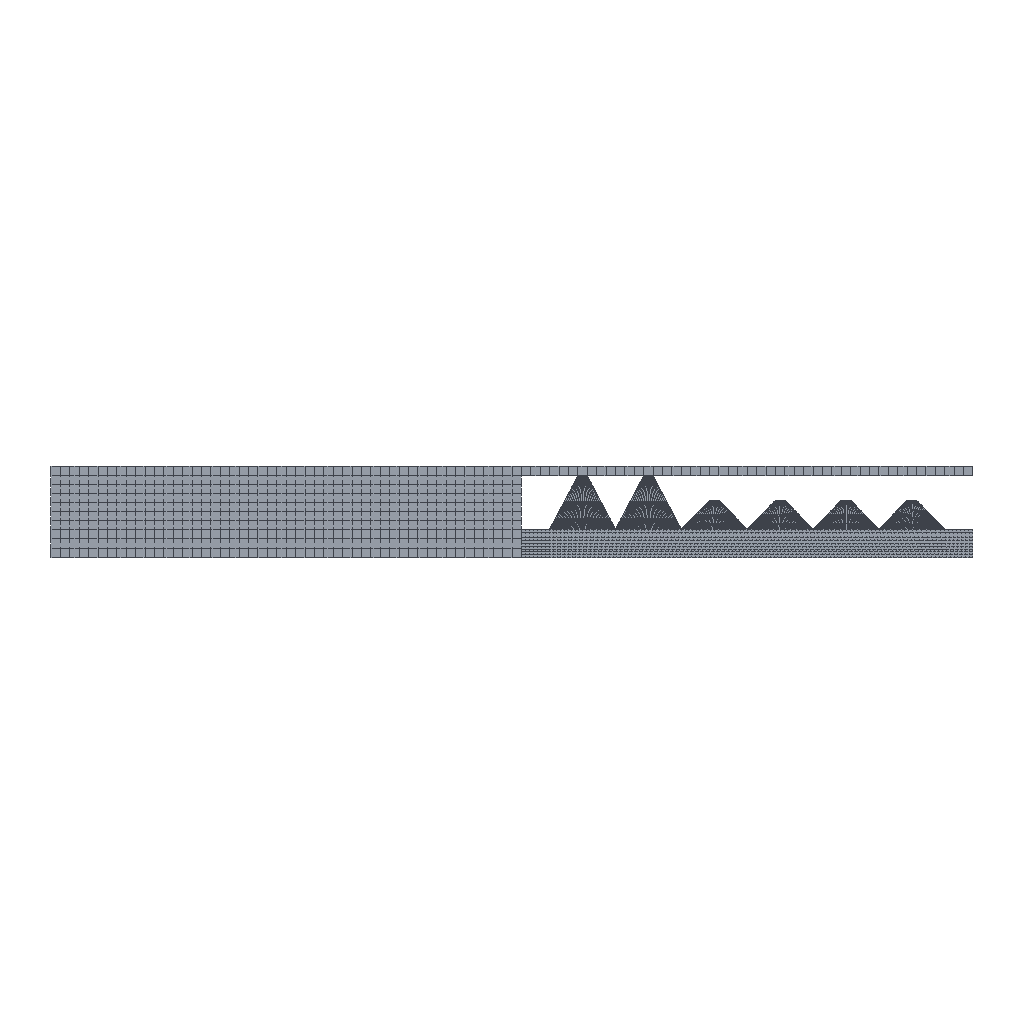Simulation study | abaqus
Set-up summary:
category,name,step,type,value,unit,region
solver,abaqus,,Abaqus/CAE 2024
units,unstated,,unstated,E=45 density=1.05e-09 (no match)
analysis,Step-1,,dynamic explicit,nlgeom=True; time_period=1
mesh,nodes,,,17497
mesh,elements,,,16380
element_type,CPS4R,,,16380
material,PDMS,,E,45
material,PDMS,,nu,0.45
material,PDMS,,density,1.05e-09
material,PI,,E,2500
material,PI,,nu,0.34
material,PI,,density,1.42e-09
material,pu,,E,30
material,pu,,nu,0.48
material,pu,,density,1.25e-09
section,PI,,solid section,,,Set-1
section,pu,,solid section,,,_PickedSet2
section,PDMS,,solid section,,,Set-9
load,Load-1,Step-1,pressure,0.5,,_PickedSurf165
bc,BC-1,Step-1,pinned,[dofs=PINNED],,_PickedSet166
bc,BC-2,Step-1,xsymm,[dofs=XSYMM],,_PickedSet167
contact,Constraint-1,initial,tie,,,_PickedSurf129 / _PickedSurf130
contact,Constraint-2,initial,tie,,,_PickedSurf158 / _PickedSurf157
contact,Int-2,Step-1,contact pair,interaction=IntProp-1; friction=0; behavior=hard,,_PickedSurf168 / _PickedSurf169
Abaqus input file, long lists of numbers shortened:
*Heading
** Job name: deck Model name: Model-E-05
** Generated by: Abaqus/CAE 2024
*Preprint, echo=NO, model=NO, history=NO, contact=NO
**
** PARTS
**
*Part, name=Part-2
*Node
      1,          5.5,  0.9
      2,          5.5,           1.
** (196 more lines like these left out)
*Element, type=CPS4R
 1,   1,   2,   7, 104
 2, 104,   7,   8, 103
** (96 more lines like these left out)
*Nset, nset=Set-1, generate
   1,  198,    1
*Elset, elset=Set-1, generate
  1,  98,   1
** Section: rigid
*Solid Section, elset=Set-1, material=PI
,
*End Part
**
*Part, name=Part-3
*Node
      1,           0.,  0.3
      2,          -5.,  0.3
** (508 more lines like these left out)
*Element, type=CPS4R
  1,   1,   7, 168, 108
  2,   7,   8, 169, 168
** (448 more lines like these left out)
*Nset, nset=_PickedSet2, internal, generate
   1,  510,    1
*Elset, elset=_PickedSet2, internal, generate
   1,  450,    1
** Section: PU
*Solid Section, elset=_PickedSet2, material=pu
,
*End Part
**
*Part, name=part-1
*Node
      1,   -2.1,           0.
      2,        -1.75,           0.
** (16787 more lines like these left out)
*Element, type=CPS4R
   1,    1,   37, 2833,  404
   2,   37,   38, 2834, 2833
** (15830 more lines like these left out)
*Nset, nset=Set-9, generate
     1,  16789,      1
*Elset, elset=Set-9, generate
     1,  15832,      1
** Section: PDMS
*Solid Section, elset=Set-9, material=PDMS
,
*End Part
**
**
** ASSEMBLY
**
*Assembly, name=Assembly
**
*Instance, name=Part-2-1, part=Part-2
         -3.,        -0.33,           0.
*End Instance
**
*Instance, name=part-1-1, part=part-1
         4.9,           0.,           0.
*End Instance
**
*Instance, name=Part-3-1, part=Part-3
         2.5,         -0.3,           0.
*End Instance
**
*Nset, nset=Set-4, instance=Part-2-1
   2,   3,   6,   7,   8,   9,  10,  11,  12,  13,  14,  15,  16,  17,  18,  19
  20,  21,  22,  23,  24,  25,  26,  27,  28,  29,  30,  31,  32,  33,  34,  35
** (5 more lines like these left out)
*Elset, elset=Set-4, instance=Part-2-1, generate
  1,  98,   1
*Nset, nset=_PickedSet166, internal, instance=part-1-1
   31,   32,   33, 2565, 2566, 2567, 2568, 2569, 2570, 2571, 2572, 2573, 2574, 2575, 2576, 2577
 2578, 2579, 2580, 2581, 2582, 2583, 2584, 2585, 2586, 2587, 2588, 2589, 2590, 2591, 2592, 2593
** (6 more lines like these left out)
*Nset, nset=_PickedSet166, internal, instance=Part-3-1
   3,   4,  58,  59,  60,  61,  62,  63,  64,  65,  66,  67,  68,  69,  70,  71
  72,  73,  74,  75,  76,  77,  78,  79,  80,  81,  82,  83,  84,  85,  86,  87
** (2 more lines like these left out)
*Elset, elset=_PickedSet166, internal, instance=part-1-1, generate
 13816,  15006,     10
*Elset, elset=_PickedSet166, internal, instance=Part-3-1, generate
 101,  150,    1
*Nset, nset=_PickedSet167, internal, instance=Part-2-1
 5, 6
*Nset, nset=_PickedSet167, internal, instance=part-1-1
   33,   35, 2683, 2684, 2685, 2686, 2687, 2688, 2689, 2690, 2691
*Elset, elset=_PickedSet167, internal, instance=Part-2-1
 98,
*Elset, elset=_PickedSet167, internal, instance=part-1-1, generate
 14997,  15006,      1
*Elset, elset=_Surf-3_S2, internal, instance=Part-2-1, generate
 51,  98,   1
*Elset, elset=_Surf-3_S2, internal, instance=Part-3-1, generate
 200,  450,   50
*Elset, elset=_Surf-3_S4, internal, instance=part-1-1
 13807, 13817, 13827, 13837, 13847, 13857, 13867, 14937, 14947, 14957, 14967, 14977, 14987, 14997
*Surface, type=ELEMENT, name=Surf-3
_Surf-3_S2, S2
_Surf-3_S4, S4
*Elset, elset=__PickedSurf129_S3, internal, instance=Part-3-1, generate
 401,  450,    1
*Surface, type=ELEMENT, name=_PickedSurf129, internal
__PickedSurf129_S3, S3
*Elset, elset=__PickedSurf130_S4, internal, instance=Part-2-1, generate
  1,  50,   1
*Elset, elset=__PickedSurf130_S2, internal, instance=Part-2-1, generate
 51,  98,   1
*Surface, type=ELEMENT, name=_PickedSurf130, internal
__PickedSurf130_S4, S4
__PickedSurf130_S2, S2
*Elset, elset=__PickedSurf157_S4, internal, instance=Part-3-1, generate
   1,  101,   50
*Surface, type=ELEMENT, name=_PickedSurf157, internal
__PickedSurf157_S4, S4
*Elset, elset=__PickedSurf158_S1, internal, instance=part-1-1, generate
 13807,  13816,      1
*Surface, type=ELEMENT, name=_PickedSurf158, internal
__PickedSurf158_S1, S1
*Elset, elset=__PickedSurf165_S2, internal, instance=Part-2-1, generate
  1,  50,   1
*Elset, elset=__PickedSurf165_S4, internal, instance=Part-2-1, generate
 51,  98,   1
*Surface, type=ELEMENT, name=_PickedSurf165, internal
__PickedSurf165_S2, S2
__PickedSurf165_S4, S4
*Elset, elset=__PickedSurf168_S2, internal, instance=Part-2-1, generate
 51,  98,   1
*Surface, type=ELEMENT, name=_PickedSurf168, internal
__PickedSurf168_S2, S2
*Elset, elset=__PickedSurf169_S3, internal, instance=part-1-1
  1585,  1586,  1587,  1588,  1589,  1590,  1591,  1592,  1593,  3010,  3011,  3012,  3013,  3014,  3015,  3016
  3017,  3018,  3019,  3020,  3021,  3022,  3023,  3024,  3025,  3026,  3027,  3028,  3029,  3030,  3031,  3032
** (53 more lines like these left out)
*Elset, elset=__PickedSurf169_S4, internal, instance=part-1-1
     1,    10,    19,    28,    37,    46,    55,    64,    73,    82,    91,   100,   109,   118,   127,   136
   145,   154,   163,   172,   181,   190,   199,   208,   217,   226,   235,   244,   253,   262,   271,   280
** (11 more lines like these left out)
*Elset, elset=__PickedSurf169_S2, internal, instance=part-1-1
  3363,  3540,  3717,  3894,  4071,  4248,  4425,  4602,  4779,  4788,  4797,  4806,  4815,  4824,  4833,  4842
  4851,  4860,  4869,  4878,  4887,  4896,  4905,  4914,  4923,  4932,  4941,  4950,  4959,  4968,  4977,  4986
** (42 more lines like these left out)
*Surface, type=ELEMENT, name=_PickedSurf169, internal
__PickedSurf169_S3, S3
__PickedSurf169_S4, S4
__PickedSurf169_S2, S2
** Constraint: Constraint-1
*Tie, name=Constraint-1, adjust=yes, no thickness
_PickedSurf129, _PickedSurf130
** Constraint: Constraint-2
*Tie, name=Constraint-2, adjust=yes, no thickness
_PickedSurf158, _PickedSurf157
*End Assembly
*Amplitude, name=Amp-1, definition=EQUALLY SPACED, fixed interval=1.
             0.,              1.
**
** MATERIALS
**
*Material, name=PDMS
*Density
 1.05e-09,
*Elastic
45., 0.45
*Material, name=PI
*Density
 1.42e-09,
*Elastic
2500., 0.34
*Material, name=pu
*Density
 1.25e-09,
*Elastic
30., 0.48
**
** INTERACTION PROPERTIES
**
*Surface Interaction, name=IntProp-1
*Friction
0.,
*Surface Behavior, pressure-overclosure=HARD
** ----------------------------------------------------------------
**
** STEP: Step-1
**
*Step, name=Step-1, nlgeom=YES
*Dynamic, Explicit
, 1.
*Bulk Viscosity
0.06, 1.2
** Mass Scaling: Semi-Automatic
**               Whole Model
*Variable Mass Scaling, dt=1e-05, type=below min, number interval=5
**
** BOUNDARY CONDITIONS
**
** Name: BC-1 Type: Symmetry/Antisymmetry/Encastre
*Boundary
_PickedSet166, PINNED
** Name: BC-2 Type: Symmetry/Antisymmetry/Encastre
*Boundary
_PickedSet167, XSYMM
**
** LOADS
**
** Name: Load-1   Type: Pressure
*Dsload, amplitude=Amp-1
_PickedSurf165, P, 0.5
**
** INTERACTIONS
**
** Interaction: Int-2
*Contact Pair, interaction=IntProp-1, mechanical constraint=KINEMATIC, cpset=Int-2
_PickedSurf168, _PickedSurf169
**
** OUTPUT REQUESTS
**
*Restart, write, number interval=1, time marks=NO
**
** FIELD OUTPUT: F-Output-1
**
*Output, field, variable=PRESELECT
**
** HISTORY OUTPUT: H-Output-1
**
*Output, history, variable=PRESELECT
*End Step
Results summary:
result,odb.job_status,,,JOB_STATUS_COMPLETED_SUCCESSFULLY,"consistent, unstated (Abaqus has no unit system)"
result,steps[0].procedure,Step-1,,"*DYNAMIC, EXPLICIT","consistent, unstated (Abaqus has no unit system)"
result,steps[0].time_period,Step-1,,1,"consistent, unstated (Abaqus has no unit system)"
result,steps[0].n_frames,Step-1,,21,"consistent, unstated (Abaqus has no unit system)"
result,steps[0].last_frame.id,Step-1,,106046,"consistent, unstated (Abaqus has no unit system)"
result,steps[0].last_frame.value,Step-1,,1,"consistent, unstated (Abaqus has no unit system)"
result,steps[0].last_frame.description,Step-1,,Increment    106046: Step Time =    1.000,"consistent, unstated (Abaqus has no unit system)"
result,steps[0].completed,Step-1,,True,"consistent, unstated (Abaqus has no unit system)"
result,steps[0].max_U_magnitude,Step-1,,0.3589,"consistent, unstated (Abaqus has no unit system)"
result,steps[0].max_S_mises,Step-1,,21.454,"consistent, unstated (Abaqus has no unit system)"
result,steps[0].RF_sum[1],Step-1,,0.2015,"consistent, unstated (Abaqus has no unit system)"
result,steps[0].RF_sum[2],Step-1,,4.86,"consistent, unstated (Abaqus has no unit system)"
result,steps[0].diagnostic.n_increments,Step-1,,21,"consistent, unstated (Abaqus has no unit system)"